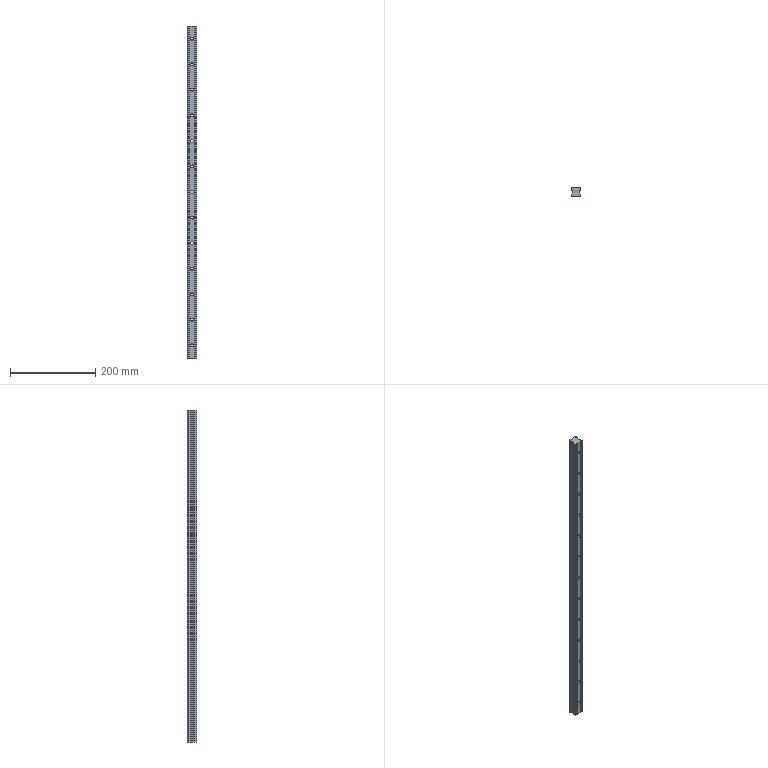Part | SolidWorks | features ICE 6, Draft 4, Chamfer 2, HoleWzd 2, Extrusion 1, LPattern 1 | 1 solid | 99 faces | box 23 x 22 x 780 mm | volume 325761 mm3 | cylinder 56 | plane 43 | commonest cylinder face diameters 7 x26 11 x26 4.6 x4